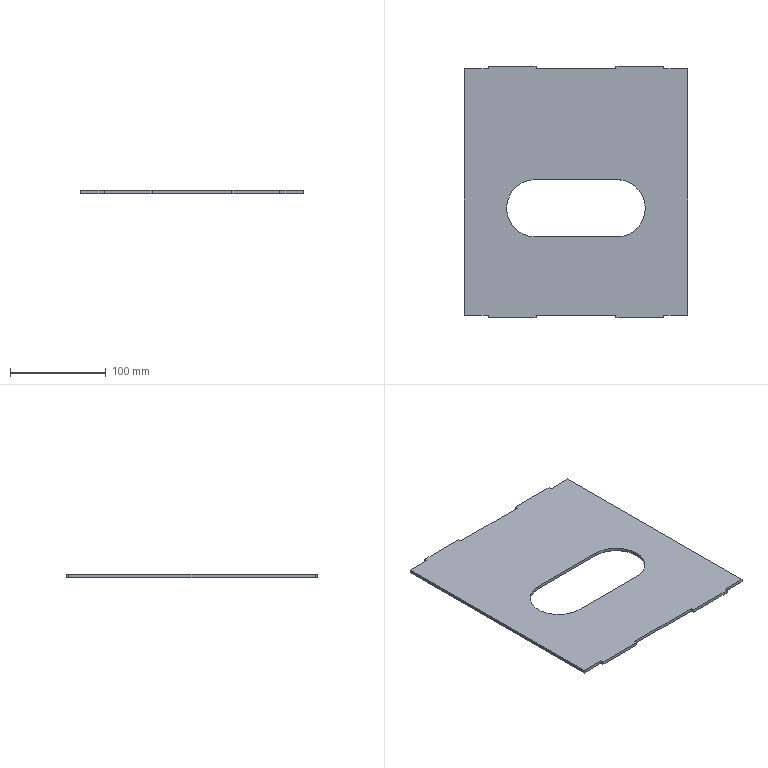Part | SolidWorks | features FlatPattern 1, SMBaseFlange 1, SheetMetal 1 | 1 solid | 27 faces | box 233.6 x 263.3 x 3.2 mm | volume 168889 mm3 | plane 24 | cylinder 3 | commonest cylinder face diameters 60 x3
STEP:
#1=CARTESIAN_POINT('',(-174.05,-276.65,-3.2));
#2=VERTEX_POINT('',#1);
#3=CARTESIAN_POINT('',(-204.05,-246.65,-3.2));
#4=VERTEX_POINT('',#3);
#5=CARTESIAN_POINT('',(-204.05,-276.65,-3.2));
#6=DIRECTION('',(0.,0.,1.));
#7=DIRECTION('',(1.,0.,0.));
#8=AXIS2_PLACEMENT_3D('',#5,#6,#7);
#9=CIRCLE('',#8,30.);
#10=EDGE_CURVE('',#2,#4,#9,.T.);
#11=ORIENTED_EDGE('',*,*,#10,.F.);
#12=CARTESIAN_POINT('',(-174.05,-276.65,0.));
#13=VERTEX_POINT('',#12);
#14=CARTESIAN_POINT('',(-174.05,-276.65,-3.2));
#15=DIRECTION('',(0.,0.,1.));
#16=VECTOR('',#15,1000.);
#17=LINE('',#14,#16);
#18=EDGE_CURVE('',#2,#13,#17,.T.);
#19=ORIENTED_EDGE('',*,*,#18,.T.);
#20=CARTESIAN_POINT('',(-204.05,-246.65,0.));
#21=VERTEX_POINT('',#20);
#22=CARTESIAN_POINT('',(-204.05,-276.65,0.));
#23=DIRECTION('',(0.,0.,1.));
#24=DIRECTION('',(1.,0.,0.));
#25=AXIS2_PLACEMENT_3D('',#22,#23,#24);
#26=CIRCLE('',#25,30.);
#27=EDGE_CURVE('',#13,#21,#26,.T.);
#28=ORIENTED_EDGE('',*,*,#27,.T.);
#29=CARTESIAN_POINT('',(-204.05,-246.65,-3.2));
#30=DIRECTION('',(0.,0.,1.));
#31=VECTOR('',#30,1000.);
#32=LINE('',#29,#31);
#33=EDGE_CURVE('',#4,#21,#32,.T.);
#34=ORIENTED_EDGE('',*,*,#33,.F.);
#35=EDGE_LOOP('',(#11,#19,#28,#34));
#36=FACE_OUTER_BOUND('',#35,.T.);
#37=CARTESIAN_POINT('',(-204.05,-276.65,-3.2));
#38=DIRECTION('',(0.,0.,1.));
#39=DIRECTION('',(1.,0.,0.));
#40=AXIS2_PLACEMENT_3D('',#37,#38,#39);
#41=CYLINDRICAL_SURFACE('',#40,30.);
#42=ADVANCED_FACE('',(#36),#41,.F.);
#43=CARTESIAN_POINT('',(-129.75,-388.35,0.));
#44=VERTEX_POINT('',#43);
#45=CARTESIAN_POINT('',(-129.75,-131.05,0.));
#46=VERTEX_POINT('',#45);
#47=CARTESIAN_POINT('',(-129.75,-388.35,0.));
#48=DIRECTION('',(0.,1.,0.));
#49=VECTOR('',#48,1000.);
#50=LINE('',#47,#49);
#51=EDGE_CURVE('',#44,#46,#50,.T.);
#52=ORIENTED_EDGE('',*,*,#51,.F.);
#53=CARTESIAN_POINT('',(-129.75,-388.35,-3.2));
#54=VERTEX_POINT('',#53);
#55=CARTESIAN_POINT('',(-129.75,-388.35,-3.2));
#56=DIRECTION('',(0.,0.,1.));
#57=VECTOR('',#56,1000.);
#58=LINE('',#55,#57);
#59=EDGE_CURVE('',#54,#44,#58,.T.);
#60=ORIENTED_EDGE('',*,*,#59,.F.);
#61=CARTESIAN_POINT('',(-129.75,-131.05,-3.2));
#62=VERTEX_POINT('',#61);
#63=CARTESIAN_POINT('',(-129.75,-388.35,-3.2));
#64=DIRECTION('',(0.,1.,0.));
#65=VECTOR('',#64,1000.);
#66=LINE('',#63,#65);
#67=EDGE_CURVE('',#54,#62,#66,.T.);
#68=ORIENTED_EDGE('',*,*,#67,.T.);
#69=CARTESIAN_POINT('',(-129.75,-131.05,-3.2));
#70=DIRECTION('',(0.,0.,1.));
#71=VECTOR('',#70,1000.);
#72=LINE('',#69,#71);
#73=EDGE_CURVE('',#62,#46,#72,.T.);
#74=ORIENTED_EDGE('',*,*,#73,.T.);
#75=EDGE_LOOP('',(#52,#60,#68,#74));
#76=FACE_OUTER_BOUND('',#75,.T.);
#77=CARTESIAN_POINT('',(-129.75,-388.35,-3.2));
#78=DIRECTION('',(1.,0.,0.));
#79=DIRECTION('',(0.,0.,-1.));
#80=AXIS2_PLACEMENT_3D('',#77,#78,#79);
#81=PLANE('',#80);
#82=ADVANCED_FACE('',(#76),#81,.T.);
#83=CARTESIAN_POINT('',(-154.75,-388.35,0.));
#84=VERTEX_POINT('',#83);
#85=CARTESIAN_POINT('',(-129.75,-388.35,0.));
#86=DIRECTION('',(1.,0.,0.));
#87=VECTOR('',#86,1000.);
#88=LINE('',#85,#87);
#89=EDGE_CURVE('',#84,#44,#88,.T.);
#90=ORIENTED_EDGE('',*,*,#89,.F.);
#91=CARTESIAN_POINT('',(-154.75,-388.35,-3.2));
#92=VERTEX_POINT('',#91);
#93=CARTESIAN_POINT('',(-154.75,-388.35,-3.2));
#94=DIRECTION('',(0.,0.,1.));
#95=VECTOR('',#94,1000.);
#96=LINE('',#93,#95);
#97=EDGE_CURVE('',#92,#84,#96,.T.);
#98=ORIENTED_EDGE('',*,*,#97,.F.);
#99=CARTESIAN_POINT('',(-129.75,-388.35,-3.2));
#100=DIRECTION('',(1.,0.,0.));
#101=VECTOR('',#100,1000.);
#102=LINE('',#99,#101);
#103=EDGE_CURVE('',#92,#54,#102,.T.);
#104=ORIENTED_EDGE('',*,*,#103,.T.);
#105=ORIENTED_EDGE('',*,*,#59,.T.);
#106=EDGE_LOOP('',(#90,#98,#104,#105));
#107=FACE_OUTER_BOUND('',#106,.T.);
#108=CARTESIAN_POINT('',(-129.75,-388.35,-3.2));
#109=DIRECTION('',(0.,-1.,0.));
#110=DIRECTION('',(0.,0.,-1.));
#111=AXIS2_PLACEMENT_3D('',#108,#109,#110);
#112=PLANE('',#111);
#113=ADVANCED_FACE('',(#107),#112,.T.);
#114=CARTESIAN_POINT('',(-154.75,-391.35,0.));
#115=VERTEX_POINT('',#114);
#116=CARTESIAN_POINT('',(-154.75,-388.35,0.));
#117=DIRECTION('',(0.,1.,0.));
#118=VECTOR('',#117,1000.);
#119=LINE('',#116,#118);
#120=EDGE_CURVE('',#115,#84,#119,.T.);
#121=ORIENTED_EDGE('',*,*,#120,.F.);
#122=CARTESIAN_POINT('',(-154.75,-391.35,-3.2));
#123=VERTEX_POINT('',#122);
#124=CARTESIAN_POINT('',(-154.75,-391.35,-3.2));
#125=DIRECTION('',(0.,0.,1.));
#126=VECTOR('',#125,1000.);
#127=LINE('',#124,#126);
#128=EDGE_CURVE('',#123,#115,#127,.T.);
#129=ORIENTED_EDGE('',*,*,#128,.F.);
#130=CARTESIAN_POINT('',(-154.75,-388.35,-3.2));
#131=DIRECTION('',(0.,1.,0.));
#132=VECTOR('',#131,1000.);
#133=LINE('',#130,#132);
#134=EDGE_CURVE('',#123,#92,#133,.T.);
#135=ORIENTED_EDGE('',*,*,#134,.T.);
#136=ORIENTED_EDGE('',*,*,#97,.T.);
#137=EDGE_LOOP('',(#121,#129,#135,#136));
#138=FACE_OUTER_BOUND('',#137,.T.);
#139=CARTESIAN_POINT('',(-154.75,-388.35,-3.2));
#140=DIRECTION('',(1.,0.,0.));
#141=DIRECTION('',(0.,0.,-1.));
#142=AXIS2_PLACEMENT_3D('',#139,#140,#141);
#143=PLANE('',#142);
#144=ADVANCED_FACE('',(#138),#143,.T.);
#145=CARTESIAN_POINT('',(-204.75,-391.35,0.));
#146=VERTEX_POINT('',#145);
#147=CARTESIAN_POINT('',(-154.75,-391.35,0.));
#148=DIRECTION('',(1.,0.,0.));
#149=VECTOR('',#148,1000.);
#150=LINE('',#147,#149);
#151=EDGE_CURVE('',#146,#115,#150,.T.);
#152=ORIENTED_EDGE('',*,*,#151,.F.);
#153=CARTESIAN_POINT('',(-204.75,-391.35,-3.2));
#154=VERTEX_POINT('',#153);
#155=CARTESIAN_POINT('',(-204.75,-391.35,-3.2));
#156=DIRECTION('',(0.,0.,1.));
#157=VECTOR('',#156,1000.);
#158=LINE('',#155,#157);
#159=EDGE_CURVE('',#154,#146,#158,.T.);
#160=ORIENTED_EDGE('',*,*,#159,.F.);
#161=CARTESIAN_POINT('',(-154.75,-391.35,-3.2));
#162=DIRECTION('',(1.,0.,0.));
#163=VECTOR('',#162,1000.);
#164=LINE('',#161,#163);
#165=EDGE_CURVE('',#154,#123,#164,.T.);
#166=ORIENTED_EDGE('',*,*,#165,.T.);
#167=ORIENTED_EDGE('',*,*,#128,.T.);
#168=EDGE_LOOP('',(#152,#160,#166,#167));
#169=FACE_OUTER_BOUND('',#168,.T.);
#170=CARTESIAN_POINT('',(-154.75,-391.35,-3.2));
#171=DIRECTION('',(0.,-1.,0.));
#172=DIRECTION('',(0.,0.,-1.));
#173=AXIS2_PLACEMENT_3D('',#170,#171,#172);
#174=PLANE('',#173);
#175=ADVANCED_FACE('',(#169),#174,.T.);
#176=CARTESIAN_POINT('',(-204.75,-388.35,0.));
#177=VERTEX_POINT('',#176);
#178=CARTESIAN_POINT('',(-204.75,-391.35,0.));
#179=DIRECTION('',(0.,-1.,0.));
#180=VECTOR('',#179,1000.);
#181=LINE('',#178,#180);
#182=EDGE_CURVE('',#177,#146,#181,.T.);
#183=ORIENTED_EDGE('',*,*,#182,.F.);
#184=CARTESIAN_POINT('',(-204.75,-388.35,-3.2));
#185=VERTEX_POINT('',#184);
#186=CARTESIAN_POINT('',(-204.75,-388.35,-3.2));
#187=DIRECTION('',(0.,0.,1.));
#188=VECTOR('',#187,1000.);
#189=LINE('',#186,#188);
#190=EDGE_CURVE('',#185,#177,#189,.T.);
#191=ORIENTED_EDGE('',*,*,#190,.F.);
#192=CARTESIAN_POINT('',(-204.75,-391.35,-3.2));
#193=DIRECTION('',(0.,-1.,0.));
#194=VECTOR('',#193,1000.);
#195=LINE('',#192,#194);
#196=EDGE_CURVE('',#185,#154,#195,.T.);
#197=ORIENTED_EDGE('',*,*,#196,.T.);
#198=ORIENTED_EDGE('',*,*,#159,.T.);
#199=EDGE_LOOP('',(#183,#191,#197,#198));
#200=FACE_OUTER_BOUND('',#199,.T.);
#201=CARTESIAN_POINT('',(-204.75,-391.35,-3.2));
#202=DIRECTION('',(-1.,0.,0.));
#203=DIRECTION('',(0.,0.,1.));
#204=AXIS2_PLACEMENT_3D('',#201,#202,#203);
#205=PLANE('',#204);
#206=ADVANCED_FACE('',(#200),#205,.T.);
#207=CARTESIAN_POINT('',(-288.35,-388.35,0.));
#208=VERTEX_POINT('',#207);
#209=CARTESIAN_POINT('',(-204.75,-388.35,0.));
#210=DIRECTION('',(1.,0.,0.));
#211=VECTOR('',#210,1000.);
#212=LINE('',#209,#211);
#213=EDGE_CURVE('',#208,#177,#212,.T.);
#214=ORIENTED_EDGE('',*,*,#213,.F.);
#215=CARTESIAN_POINT('',(-288.35,-388.35,-3.2));
#216=VERTEX_POINT('',#215);
#217=CARTESIAN_POINT('',(-288.35,-388.35,-3.2));
#218=DIRECTION('',(0.,0.,1.));
#219=VECTOR('',#218,1000.);
#220=LINE('',#217,#219);
#221=EDGE_CURVE('',#216,#208,#220,.T.);
#222=ORIENTED_EDGE('',*,*,#221,.F.);
#223=CARTESIAN_POINT('',(-204.75,-388.35,-3.2));
#224=DIRECTION('',(1.,0.,0.));
#225=VECTOR('',#224,1000.);
#226=LINE('',#223,#225);
#227=EDGE_CURVE('',#216,#185,#226,.T.);
#228=ORIENTED_EDGE('',*,*,#227,.T.);
#229=ORIENTED_EDGE('',*,*,#190,.T.);
#230=EDGE_LOOP('',(#214,#222,#228,#229));
#231=FACE_OUTER_BOUND('',#230,.T.);
#232=CARTESIAN_POINT('',(-204.75,-388.35,-3.2));
#233=DIRECTION('',(0.,-1.,0.));
#234=DIRECTION('',(0.,0.,-1.));
#235=AXIS2_PLACEMENT_3D('',#232,#233,#234);
#236=PLANE('',#235);
#237=ADVANCED_FACE('',(#231),#236,.T.);
#238=CARTESIAN_POINT('',(-288.35,-391.35,0.));
#239=VERTEX_POINT('',#238);
#240=CARTESIAN_POINT('',(-288.35,-391.35,0.));
#241=DIRECTION('',(0.,1.,0.));
#242=VECTOR('',#241,1000.);
#243=LINE('',#240,#242);
#244=EDGE_CURVE('',#239,#208,#243,.T.);
#245=ORIENTED_EDGE('',*,*,#244,.F.);
#246=CARTESIAN_POINT('',(-288.35,-391.35,-3.2));
#247=VERTEX_POINT('',#246);
#248=CARTESIAN_POINT('',(-288.35,-391.35,-3.2));
#249=DIRECTION('',(0.,0.,1.));
#250=VECTOR('',#249,1000.);
#251=LINE('',#248,#250);
#252=EDGE_CURVE('',#247,#239,#251,.T.);
#253=ORIENTED_EDGE('',*,*,#252,.F.);
#254=CARTESIAN_POINT('',(-288.35,-391.35,-3.2));
#255=DIRECTION('',(0.,1.,0.));
#256=VECTOR('',#255,1000.);
#257=LINE('',#254,#256);
#258=EDGE_CURVE('',#247,#216,#257,.T.);
#259=ORIENTED_EDGE('',*,*,#258,.T.);
#260=ORIENTED_EDGE('',*,*,#221,.T.);
#261=EDGE_LOOP('',(#245,#253,#259,#260));
#262=FACE_OUTER_BOUND('',#261,.T.);
#263=CARTESIAN_POINT('',(-288.35,-391.35,-3.2));
#264=DIRECTION('',(1.,0.,0.));
#265=DIRECTION('',(0.,0.,-1.));
#266=AXIS2_PLACEMENT_3D('',#263,#264,#265);
#267=PLANE('',#266);
#268=ADVANCED_FACE('',(#262),#267,.T.);
#269=CARTESIAN_POINT('',(-338.35,-391.35,0.));
#270=VERTEX_POINT('',#269);
#271=CARTESIAN_POINT('',(-338.35,-391.35,0.));
#272=DIRECTION('',(1.,0.,0.));
#273=VECTOR('',#272,1000.);
#274=LINE('',#271,#273);
#275=EDGE_CURVE('',#270,#239,#274,.T.);
#276=ORIENTED_EDGE('',*,*,#275,.F.);
#277=CARTESIAN_POINT('',(-338.35,-391.35,-3.2));
#278=VERTEX_POINT('',#277);
#279=CARTESIAN_POINT('',(-338.35,-391.35,-3.2));
#280=DIRECTION('',(0.,0.,1.));
#281=VECTOR('',#280,1000.);
#282=LINE('',#279,#281);
#283=EDGE_CURVE('',#278,#270,#282,.T.);
#284=ORIENTED_EDGE('',*,*,#283,.F.);
#285=CARTESIAN_POINT('',(-338.35,-391.35,-3.2));
#286=DIRECTION('',(1.,0.,0.));
#287=VECTOR('',#286,1000.);
#288=LINE('',#285,#287);
#289=EDGE_CURVE('',#278,#247,#288,.T.);
#290=ORIENTED_EDGE('',*,*,#289,.T.);
#291=ORIENTED_EDGE('',*,*,#252,.T.);
#292=EDGE_LOOP('',(#276,#284,#290,#291));
#293=FACE_OUTER_BOUND('',#292,.T.);
#294=CARTESIAN_POINT('',(-338.35,-391.35,-3.2));
#295=DIRECTION('',(0.,-1.,0.));
#296=DIRECTION('',(0.,0.,-1.));
#297=AXIS2_PLACEMENT_3D('',#294,#295,#296);
#298=PLANE('',#297);
#299=ADVANCED_FACE('',(#293),#298,.T.);
#300=CARTESIAN_POINT('',(-338.35,-388.35,0.));
#301=VERTEX_POINT('',#300);
#302=CARTESIAN_POINT('',(-338.35,-388.35,0.));
#303=DIRECTION('',(0.,-1.,0.));
#304=VECTOR('',#303,1000.);
#305=LINE('',#302,#304);
#306=EDGE_CURVE('',#301,#270,#305,.T.);
#307=ORIENTED_EDGE('',*,*,#306,.F.);
#308=CARTESIAN_POINT('',(-338.35,-388.35,-3.2));
#309=VERTEX_POINT('',#308);
#310=CARTESIAN_POINT('',(-338.35,-388.35,-3.2));
#311=DIRECTION('',(0.,0.,1.));
#312=VECTOR('',#311,1000.);
#313=LINE('',#310,#312);
#314=EDGE_CURVE('',#309,#301,#313,.T.);
#315=ORIENTED_EDGE('',*,*,#314,.F.);
#316=CARTESIAN_POINT('',(-338.35,-388.35,-3.2));
#317=DIRECTION('',(0.,-1.,0.));
#318=VECTOR('',#317,1000.);
#319=LINE('',#316,#318);
#320=EDGE_CURVE('',#309,#278,#319,.T.);
#321=ORIENTED_EDGE('',*,*,#320,.T.);
#322=ORIENTED_EDGE('',*,*,#283,.T.);
#323=EDGE_LOOP('',(#307,#315,#321,#322));
#324=FACE_OUTER_BOUND('',#323,.T.);
#325=CARTESIAN_POINT('',(-338.35,-388.35,-3.2));
#326=DIRECTION('',(-1.,0.,0.));
#327=DIRECTION('',(0.,0.,1.));
#328=AXIS2_PLACEMENT_3D('',#325,#326,#327);
#329=PLANE('',#328);
#330=ADVANCED_FACE('',(#324),#329,.T.);
#331=CARTESIAN_POINT('',(-363.35,-388.35,0.));
#332=VERTEX_POINT('',#331);
#333=CARTESIAN_POINT('',(-338.35,-388.35,0.));
#334=DIRECTION('',(1.,0.,0.));
#335=VECTOR('',#334,1000.);
#336=LINE('',#333,#335);
#337=EDGE_CURVE('',#332,#301,#336,.T.);
#338=ORIENTED_EDGE('',*,*,#337,.F.);
#339=CARTESIAN_POINT('',(-363.35,-388.35,-3.2));
#340=VERTEX_POINT('',#339);
#341=CARTESIAN_POINT('',(-363.35,-388.35,-3.2));
#342=DIRECTION('',(0.,0.,1.));
#343=VECTOR('',#342,1000.);
#344=LINE('',#341,#343);
#345=EDGE_CURVE('',#340,#332,#344,.T.);
#346=ORIENTED_EDGE('',*,*,#345,.F.);
#347=CARTESIAN_POINT('',(-338.35,-388.35,-3.2));
#348=DIRECTION('',(1.,0.,0.));
#349=VECTOR('',#348,1000.);
#350=LINE('',#347,#349);
#351=EDGE_CURVE('',#340,#309,#350,.T.);
#352=ORIENTED_EDGE('',*,*,#351,.T.);
#353=ORIENTED_EDGE('',*,*,#314,.T.);
#354=EDGE_LOOP('',(#338,#346,#352,#353));
#355=FACE_OUTER_BOUND('',#354,.T.);
#356=CARTESIAN_POINT('',(-338.35,-388.35,-3.2));
#357=DIRECTION('',(0.,-1.,0.));
#358=DIRECTION('',(0.,0.,-1.));
#359=AXIS2_PLACEMENT_3D('',#356,#357,#358);
#360=PLANE('',#359);
#361=ADVANCED_FACE('',(#355),#360,.T.);
#362=CARTESIAN_POINT('',(-363.35,-131.05,0.));
#363=VERTEX_POINT('',#362);
#364=CARTESIAN_POINT('',(-363.35,-388.35,0.));
#365=DIRECTION('',(0.,-1.,0.));
#366=VECTOR('',#365,1000.);
#367=LINE('',#364,#366);
#368=EDGE_CURVE('',#363,#332,#367,.T.);
#369=ORIENTED_EDGE('',*,*,#368,.F.);
#370=CARTESIAN_POINT('',(-363.35,-131.05,-3.2));
#371=VERTEX_POINT('',#370);
#372=CARTESIAN_POINT('',(-363.35,-131.05,-3.2));
#373=DIRECTION('',(0.,0.,1.));
#374=VECTOR('',#373,1000.);
#375=LINE('',#372,#374);
#376=EDGE_CURVE('',#371,#363,#375,.T.);
#377=ORIENTED_EDGE('',*,*,#376,.F.);
#378=CARTESIAN_POINT('',(-363.35,-388.35,-3.2));
#379=DIRECTION('',(0.,-1.,0.));
#380=VECTOR('',#379,1000.);
#381=LINE('',#378,#380);
#382=EDGE_CURVE('',#371,#340,#381,.T.);
#383=ORIENTED_EDGE('',*,*,#382,.T.);
#384=ORIENTED_EDGE('',*,*,#345,.T.);
#385=EDGE_LOOP('',(#369,#377,#383,#384));
#386=FACE_OUTER_BOUND('',#385,.T.);
#387=CARTESIAN_POINT('',(-363.35,-388.35,-3.2));
#388=DIRECTION('',(-1.,0.,0.));
#389=DIRECTION('',(0.,0.,1.));
#390=AXIS2_PLACEMENT_3D('',#387,#388,#389);
#391=PLANE('',#390);
#392=ADVANCED_FACE('',(#386),#391,.T.);
#393=CARTESIAN_POINT('',(-338.35,-131.05,0.));
#394=VERTEX_POINT('',#393);
#395=CARTESIAN_POINT('',(-338.35,-131.05,0.));
#396=DIRECTION('',(-1.,0.,0.));
#397=VECTOR('',#396,1000.);
#398=LINE('',#395,#397);
#399=EDGE_CURVE('',#394,#363,#398,.T.);
#400=ORIENTED_EDGE('',*,*,#399,.F.);
#401=CARTESIAN_POINT('',(-338.35,-131.05,-3.2));
#402=VERTEX_POINT('',#401);
#403=CARTESIAN_POINT('',(-338.35,-131.05,-3.2));
#404=DIRECTION('',(0.,0.,1.));
#405=VECTOR('',#404,1000.);
#406=LINE('',#403,#405);
#407=EDGE_CURVE('',#402,#394,#406,.T.);
#408=ORIENTED_EDGE('',*,*,#407,.F.);
#409=CARTESIAN_POINT('',(-338.35,-131.05,-3.2));
#410=DIRECTION('',(-1.,0.,0.));
#411=VECTOR('',#410,1000.);
#412=LINE('',#409,#411);
#413=EDGE_CURVE('',#402,#371,#412,.T.);
#414=ORIENTED_EDGE('',*,*,#413,.T.);
#415=ORIENTED_EDGE('',*,*,#376,.T.);
#416=EDGE_LOOP('',(#400,#408,#414,#415));
#417=FACE_OUTER_BOUND('',#416,.T.);
#418=CARTESIAN_POINT('',(-338.35,-131.05,-3.2));
#419=DIRECTION('',(0.,1.,0.));
#420=DIRECTION('',(0.,0.,1.));
#421=AXIS2_PLACEMENT_3D('',#418,#419,#420);
#422=PLANE('',#421);
#423=ADVANCED_FACE('',(#417),#422,.T.);
#424=CARTESIAN_POINT('',(-338.35,-128.05,0.));
#425=VERTEX_POINT('',#424);
#426=CARTESIAN_POINT('',(-338.35,-131.05,0.));
#427=DIRECTION('',(0.,-1.,0.));
#428=VECTOR('',#427,1000.);
#429=LINE('',#426,#428);
#430=EDGE_CURVE('',#425,#394,#429,.T.);
#431=ORIENTED_EDGE('',*,*,#430,.F.);
#432=CARTESIAN_POINT('',(-338.35,-128.05,-3.2));
#433=VERTEX_POINT('',#432);
#434=CARTESIAN_POINT('',(-338.35,-128.05,-3.2));
#435=DIRECTION('',(0.,0.,1.));
#436=VECTOR('',#435,1000.);
#437=LINE('',#434,#436);
#438=EDGE_CURVE('',#433,#425,#437,.T.);
#439=ORIENTED_EDGE('',*,*,#438,.F.);
#440=CARTESIAN_POINT('',(-338.35,-131.05,-3.2));
#441=DIRECTION('',(0.,-1.,0.));
#442=VECTOR('',#441,1000.);
#443=LINE('',#440,#442);
#444=EDGE_CURVE('',#433,#402,#443,.T.);
#445=ORIENTED_EDGE('',*,*,#444,.T.);
#446=ORIENTED_EDGE('',*,*,#407,.T.);
#447=EDGE_LOOP('',(#431,#439,#445,#446));
#448=FACE_OUTER_BOUND('',#447,.T.);
#449=CARTESIAN_POINT('',(-338.35,-131.05,-3.2));
#450=DIRECTION('',(-1.,0.,0.));
#451=DIRECTION('',(0.,0.,1.));
#452=AXIS2_PLACEMENT_3D('',#449,#450,#451);
#453=PLANE('',#452);
#454=ADVANCED_FACE('',(#448),#453,.T.);
#455=CARTESIAN_POINT('',(-288.35,-128.05,0.));
#456=VERTEX_POINT('',#455);
#457=CARTESIAN_POINT('',(-338.35,-128.05,0.));
#458=DIRECTION('',(-1.,0.,0.));
#459=VECTOR('',#458,1000.);
#460=LINE('',#457,#459);
#461=EDGE_CURVE('',#456,#425,#460,.T.);
#462=ORIENTED_EDGE('',*,*,#461,.F.);
#463=CARTESIAN_POINT('',(-288.35,-128.05,-3.2));
#464=VERTEX_POINT('',#463);
#465=CARTESIAN_POINT('',(-288.35,-128.05,-3.2));
#466=DIRECTION('',(0.,0.,1.));
#467=VECTOR('',#466,1000.);
#468=LINE('',#465,#467);
#469=EDGE_CURVE('',#464,#456,#468,.T.);
#470=ORIENTED_EDGE('',*,*,#469,.F.);
#471=CARTESIAN_POINT('',(-338.35,-128.05,-3.2));
#472=DIRECTION('',(-1.,0.,0.));
#473=VECTOR('',#472,1000.);
#474=LINE('',#471,#473);
#475=EDGE_CURVE('',#464,#433,#474,.T.);
#476=ORIENTED_EDGE('',*,*,#475,.T.);
#477=ORIENTED_EDGE('',*,*,#438,.T.);
#478=EDGE_LOOP('',(#462,#470,#476,#477));
#479=FACE_OUTER_BOUND('',#478,.T.);
#480=CARTESIAN_POINT('',(-338.35,-128.05,-3.2));
#481=DIRECTION('',(0.,1.,0.));
#482=DIRECTION('',(0.,0.,1.));
#483=AXIS2_PLACEMENT_3D('',#480,#481,#482);
#484=PLANE('',#483);
#485=ADVANCED_FACE('',(#479),#484,.T.);
#486=CARTESIAN_POINT('',(-288.35,-131.05,0.));
#487=VERTEX_POINT('',#486);
#488=CARTESIAN_POINT('',(-288.35,-128.05,0.));
#489=DIRECTION('',(0.,1.,0.));
#490=VECTOR('',#489,1000.);
#491=LINE('',#488,#490);
#492=EDGE_CURVE('',#487,#456,#491,.T.);
#493=ORIENTED_EDGE('',*,*,#492,.F.);
#494=CARTESIAN_POINT('',(-288.35,-131.05,-3.2));
#495=VERTEX_POINT('',#494);
#496=CARTESIAN_POINT('',(-288.35,-131.05,-3.2));
#497=DIRECTION('',(0.,0.,1.));
#498=VECTOR('',#497,1000.);
#499=LINE('',#496,#498);
#500=EDGE_CURVE('',#495,#487,#499,.T.);
#501=ORIENTED_EDGE('',*,*,#500,.F.);
#502=CARTESIAN_POINT('',(-288.35,-128.05,-3.2));
#503=DIRECTION('',(0.,1.,0.));
#504=VECTOR('',#503,1000.);
#505=LINE('',#502,#504);
#506=EDGE_CURVE('',#495,#464,#505,.T.);
#507=ORIENTED_EDGE('',*,*,#506,.T.);
#508=ORIENTED_EDGE('',*,*,#469,.T.);
#509=EDGE_LOOP('',(#493,#501,#507,#508));
#510=FACE_OUTER_BOUND('',#509,.T.);
#511=CARTESIAN_POINT('',(-288.35,-128.05,-3.2));
#512=DIRECTION('',(1.,0.,0.));
#513=DIRECTION('',(0.,0.,-1.));
#514=AXIS2_PLACEMENT_3D('',#511,#512,#513);
#515=PLANE('',#514);
#516=ADVANCED_FACE('',(#510),#515,.T.);
#517=CARTESIAN_POINT('',(-204.75,-131.05,0.));
#518=VERTEX_POINT('',#517);
#519=CARTESIAN_POINT('',(-204.75,-131.05,0.));
#520=DIRECTION('',(-1.,0.,0.));
#521=VECTOR('',#520,1000.);
#522=LINE('',#519,#521);
#523=EDGE_CURVE('',#518,#487,#522,.T.);
#524=ORIENTED_EDGE('',*,*,#523,.F.);
#525=CARTESIAN_POINT('',(-204.75,-131.05,-3.2));
#526=VERTEX_POINT('',#525);
#527=CARTESIAN_POINT('',(-204.75,-131.05,-3.2));
#528=DIRECTION('',(0.,0.,1.));
#529=VECTOR('',#528,1000.);
#530=LINE('',#527,#529);
#531=EDGE_CURVE('',#526,#518,#530,.T.);
#532=ORIENTED_EDGE('',*,*,#531,.F.);
#533=CARTESIAN_POINT('',(-204.75,-131.05,-3.2));
#534=DIRECTION('',(-1.,0.,0.));
#535=VECTOR('',#534,1000.);
#536=LINE('',#533,#535);
#537=EDGE_CURVE('',#526,#495,#536,.T.);
#538=ORIENTED_EDGE('',*,*,#537,.T.);
#539=ORIENTED_EDGE('',*,*,#500,.T.);
#540=EDGE_LOOP('',(#524,#532,#538,#539));
#541=FACE_OUTER_BOUND('',#540,.T.);
#542=CARTESIAN_POINT('',(-204.75,-131.05,-3.2));
#543=DIRECTION('',(0.,1.,0.));
#544=DIRECTION('',(-1.,0.,0.));
#545=AXIS2_PLACEMENT_3D('',#542,#543,#544);
#546=PLANE('',#545);
#547=ADVANCED_FACE('',(#541),#546,.T.);
#548=CARTESIAN_POINT('',(-204.75,-128.05,0.));
#549=VERTEX_POINT('',#548);
#550=CARTESIAN_POINT('',(-204.75,-128.05,0.));
#551=DIRECTION('',(0.,-1.,0.));
#552=VECTOR('',#551,1000.);
#553=LINE('',#550,#552);
#554=EDGE_CURVE('',#549,#518,#553,.T.);
#555=ORIENTED_EDGE('',*,*,#554,.F.);
#556=CARTESIAN_POINT('',(-204.75,-128.05,-3.2));
#557=VERTEX_POINT('',#556);
#558=CARTESIAN_POINT('',(-204.75,-128.05,-3.2));
#559=DIRECTION('',(0.,0.,1.));
#560=VECTOR('',#559,1000.);
#561=LINE('',#558,#560);
#562=EDGE_CURVE('',#557,#549,#561,.T.);
#563=ORIENTED_EDGE('',*,*,#562,.F.);
#564=CARTESIAN_POINT('',(-204.75,-128.05,-3.2));
#565=DIRECTION('',(0.,-1.,0.));
#566=VECTOR('',#565,1000.);
#567=LINE('',#564,#566);
#568=EDGE_CURVE('',#557,#526,#567,.T.);
#569=ORIENTED_EDGE('',*,*,#568,.T.);
#570=ORIENTED_EDGE('',*,*,#531,.T.);
#571=EDGE_LOOP('',(#555,#563,#569,#570));
#572=FACE_OUTER_BOUND('',#571,.T.);
#573=CARTESIAN_POINT('',(-204.75,-128.05,-3.2));
#574=DIRECTION('',(-1.,0.,0.));
#575=DIRECTION('',(0.,0.,1.));
#576=AXIS2_PLACEMENT_3D('',#573,#574,#575);
#577=PLANE('',#576);
#578=ADVANCED_FACE('',(#572),#577,.T.);
#579=CARTESIAN_POINT('',(-154.75,-128.05,0.));
#580=VERTEX_POINT('',#579);
#581=CARTESIAN_POINT('',(-154.75,-128.05,0.));
#582=DIRECTION('',(-1.,0.,0.));
#583=VECTOR('',#582,1000.);
#584=LINE('',#581,#583);
#585=EDGE_CURVE('',#580,#549,#584,.T.);
#586=ORIENTED_EDGE('',*,*,#585,.F.);
#587=CARTESIAN_POINT('',(-154.75,-128.05,-3.2));
#588=VERTEX_POINT('',#587);
#589=CARTESIAN_POINT('',(-154.75,-128.05,-3.2));
#590=DIRECTION('',(0.,0.,1.));
#591=VECTOR('',#590,1000.);
#592=LINE('',#589,#591);
#593=EDGE_CURVE('',#588,#580,#592,.T.);
#594=ORIENTED_EDGE('',*,*,#593,.F.);
#595=CARTESIAN_POINT('',(-154.75,-128.05,-3.2));
#596=DIRECTION('',(-1.,0.,0.));
#597=VECTOR('',#596,1000.);
#598=LINE('',#595,#597);
#599=EDGE_CURVE('',#588,#557,#598,.T.);
#600=ORIENTED_EDGE('',*,*,#599,.T.);
#601=ORIENTED_EDGE('',*,*,#562,.T.);
#602=EDGE_LOOP('',(#586,#594,#600,#601));
#603=FACE_OUTER_BOUND('',#602,.T.);
#604=CARTESIAN_POINT('',(-154.75,-128.05,-3.2));
#605=DIRECTION('',(0.,1.,0.));
#606=DIRECTION('',(-1.,0.,0.));
#607=AXIS2_PLACEMENT_3D('',#604,#605,#606);
#608=PLANE('',#607);
#609=ADVANCED_FACE('',(#603),#608,.T.);
#610=CARTESIAN_POINT('',(-154.75,-131.05,0.));
#611=VERTEX_POINT('',#610);
#612=CARTESIAN_POINT('',(-154.75,-131.05,0.));
#613=DIRECTION('',(0.,1.,0.));
#614=VECTOR('',#613,1000.);
#615=LINE('',#612,#614);
#616=EDGE_CURVE('',#611,#580,#615,.T.);
#617=ORIENTED_EDGE('',*,*,#616,.F.);
#618=CARTESIAN_POINT('',(-154.75,-131.05,-3.2));
#619=VERTEX_POINT('',#618);
#620=CARTESIAN_POINT('',(-154.75,-131.05,-3.2));
#621=DIRECTION('',(0.,0.,1.));
#622=VECTOR('',#621,1000.);
#623=LINE('',#620,#622);
#624=EDGE_CURVE('',#619,#611,#623,.T.);
#625=ORIENTED_EDGE('',*,*,#624,.F.);
#626=CARTESIAN_POINT('',(-154.75,-131.05,-3.2));
#627=DIRECTION('',(0.,1.,0.));
#628=VECTOR('',#627,1000.);
#629=LINE('',#626,#628);
#630=EDGE_CURVE('',#619,#588,#629,.T.);
#631=ORIENTED_EDGE('',*,*,#630,.T.);
#632=ORIENTED_EDGE('',*,*,#593,.T.);
#633=EDGE_LOOP('',(#617,#625,#631,#632));
#634=FACE_OUTER_BOUND('',#633,.T.);
#635=CARTESIAN_POINT('',(-154.75,-131.05,-3.2));
#636=DIRECTION('',(1.,0.,0.));
#637=DIRECTION('',(0.,0.,-1.));
#638=AXIS2_PLACEMENT_3D('',#635,#636,#637);
#639=PLANE('',#638);
#640=ADVANCED_FACE('',(#634),#639,.T.);
#641=CARTESIAN_POINT('',(-129.75,-131.05,0.));
#642=DIRECTION('',(-1.,0.,0.));
#643=VECTOR('',#642,1000.);
#644=LINE('',#641,#643);
#645=EDGE_CURVE('',#46,#611,#644,.T.);
#646=ORIENTED_EDGE('',*,*,#645,.F.);
#647=ORIENTED_EDGE('',*,*,#73,.F.);
#648=CARTESIAN_POINT('',(-129.75,-131.05,-3.2));
#649=DIRECTION('',(-1.,0.,0.));
#650=VECTOR('',#649,1000.);
#651=LINE('',#648,#650);
#652=EDGE_CURVE('',#62,#619,#651,.T.);
#653=ORIENTED_EDGE('',*,*,#652,.T.);
#654=ORIENTED_EDGE('',*,*,#624,.T.);
#655=EDGE_LOOP('',(#646,#647,#653,#654));
#656=FACE_OUTER_BOUND('',#655,.T.);
#657=CARTESIAN_POINT('',(-129.75,-131.05,-3.2));
#658=DIRECTION('',(0.,1.,0.));
#659=DIRECTION('',(-1.,0.,0.));
#660=AXIS2_PLACEMENT_3D('',#657,#658,#659);
#661=PLANE('',#660);
#662=ADVANCED_FACE('',(#656),#661,.T.);
#663=CARTESIAN_POINT('',(-289.05,-306.65,-3.2));
#664=VERTEX_POINT('',#663);
#665=CARTESIAN_POINT('',(-204.05,-306.65,-3.2));
#666=VERTEX_POINT('',#665);
#667=CARTESIAN_POINT('',(-204.05,-306.65,-3.2));
#668=DIRECTION('',(1.,0.,0.));
#669=VECTOR('',#668,1000.);
#670=LINE('',#667,#669);
#671=EDGE_CURVE('',#664,#666,#670,.T.);
#672=ORIENTED_EDGE('',*,*,#671,.T.);
#673=CARTESIAN_POINT('',(-204.05,-276.65,-3.2));
#674=DIRECTION('',(0.,0.,1.));
#675=DIRECTION('',(1.,0.,0.));
#676=AXIS2_PLACEMENT_3D('',#673,#674,#675);
#677=CIRCLE('',#676,30.);
#678=EDGE_CURVE('',#666,#2,#677,.T.);
#679=ORIENTED_EDGE('',*,*,#678,.T.);
#680=ORIENTED_EDGE('',*,*,#10,.T.);
#681=CARTESIAN_POINT('',(-289.05,-246.65,-3.2));
#682=VERTEX_POINT('',#681);
#683=CARTESIAN_POINT('',(-204.05,-246.65,-3.2));
#684=DIRECTION('',(-1.,0.,0.));
#685=VECTOR('',#684,1000.);
#686=LINE('',#683,#685);
#687=EDGE_CURVE('',#4,#682,#686,.T.);
#688=ORIENTED_EDGE('',*,*,#687,.T.);
#689=CARTESIAN_POINT('',(-289.05,-276.65,-3.2));
#690=DIRECTION('',(0.,0.,1.));
#691=DIRECTION('',(1.,0.,0.));
#692=AXIS2_PLACEMENT_3D('',#689,#690,#691);
#693=CIRCLE('',#692,30.);
#694=EDGE_CURVE('',#682,#664,#693,.T.);
#695=ORIENTED_EDGE('',*,*,#694,.T.);
#696=EDGE_LOOP('',(#672,#679,#680,#688,#695));
#697=FACE_BOUND('',#696,.T.);
#698=ORIENTED_EDGE('',*,*,#67,.F.);
#699=ORIENTED_EDGE('',*,*,#103,.F.);
#700=ORIENTED_EDGE('',*,*,#134,.F.);
#701=ORIENTED_EDGE('',*,*,#165,.F.);
#702=ORIENTED_EDGE('',*,*,#196,.F.);
#703=ORIENTED_EDGE('',*,*,#227,.F.);
#704=ORIENTED_EDGE('',*,*,#258,.F.);
#705=ORIENTED_EDGE('',*,*,#289,.F.);
#706=ORIENTED_EDGE('',*,*,#320,.F.);
#707=ORIENTED_EDGE('',*,*,#351,.F.);
#708=ORIENTED_EDGE('',*,*,#382,.F.);
#709=ORIENTED_EDGE('',*,*,#413,.F.);
#710=ORIENTED_EDGE('',*,*,#444,.F.);
#711=ORIENTED_EDGE('',*,*,#475,.F.);
#712=ORIENTED_EDGE('',*,*,#506,.F.);
#713=ORIENTED_EDGE('',*,*,#537,.F.);
#714=ORIENTED_EDGE('',*,*,#568,.F.);
#715=ORIENTED_EDGE('',*,*,#599,.F.);
#716=ORIENTED_EDGE('',*,*,#630,.F.);
#717=ORIENTED_EDGE('',*,*,#652,.F.);
#718=EDGE_LOOP('',(#698,#699,#700,#701,#702,#703,#704,#705,#706,#707,#708,#709,#710,#711,#712,#713,#714,#715,#716,#717));
#719=FACE_OUTER_BOUND('',#718,.T.);
#720=CARTESIAN_POINT('',(0.,0.,-3.2));
#721=DIRECTION('',(0.,0.,1.));
#722=DIRECTION('',(1.,0.,0.));
#723=AXIS2_PLACEMENT_3D('',#720,#721,#722);
#724=PLANE('',#723);
#725=ADVANCED_FACE('',(#697,#719),#724,.F.);
#726=CARTESIAN_POINT('',(-204.05,-306.65,0.));
#727=VERTEX_POINT('',#726);
#728=CARTESIAN_POINT('',(-204.05,-276.65,0.));
#729=DIRECTION('',(0.,0.,1.));
#730=DIRECTION('',(1.,0.,0.));
#731=AXIS2_PLACEMENT_3D('',#728,#729,#730);
#732=CIRCLE('',#731,30.);
#733=EDGE_CURVE('',#727,#13,#732,.T.);
#734=ORIENTED_EDGE('',*,*,#733,.F.);
#735=CARTESIAN_POINT('',(-289.05,-306.65,0.));
#736=VERTEX_POINT('',#735);
#737=CARTESIAN_POINT('',(-204.05,-306.65,0.));
#738=DIRECTION('',(1.,0.,0.));
#739=VECTOR('',#738,1000.);
#740=LINE('',#737,#739);
#741=EDGE_CURVE('',#736,#727,#740,.T.);
#742=ORIENTED_EDGE('',*,*,#741,.F.);
#743=CARTESIAN_POINT('',(-289.05,-246.65,0.));
#744=VERTEX_POINT('',#743);
#745=CARTESIAN_POINT('',(-289.05,-276.65,0.));
#746=DIRECTION('',(0.,0.,1.));
#747=DIRECTION('',(1.,0.,0.));
#748=AXIS2_PLACEMENT_3D('',#745,#746,#747);
#749=CIRCLE('',#748,30.);
#750=EDGE_CURVE('',#744,#736,#749,.T.);
#751=ORIENTED_EDGE('',*,*,#750,.F.);
#752=CARTESIAN_POINT('',(-204.05,-246.65,0.));
#753=DIRECTION('',(-1.,0.,0.));
#754=VECTOR('',#753,1000.);
#755=LINE('',#752,#754);
#756=EDGE_CURVE('',#21,#744,#755,.T.);
#757=ORIENTED_EDGE('',*,*,#756,.F.);
#758=ORIENTED_EDGE('',*,*,#27,.F.);
#759=EDGE_LOOP('',(#734,#742,#751,#757,#758));
#760=FACE_BOUND('',#759,.T.);
#761=ORIENTED_EDGE('',*,*,#51,.T.);
#762=ORIENTED_EDGE('',*,*,#645,.T.);
#763=ORIENTED_EDGE('',*,*,#616,.T.);
#764=ORIENTED_EDGE('',*,*,#585,.T.);
#765=ORIENTED_EDGE('',*,*,#554,.T.);
#766=ORIENTED_EDGE('',*,*,#523,.T.);
#767=ORIENTED_EDGE('',*,*,#492,.T.);
#768=ORIENTED_EDGE('',*,*,#461,.T.);
#769=ORIENTED_EDGE('',*,*,#430,.T.);
#770=ORIENTED_EDGE('',*,*,#399,.T.);
#771=ORIENTED_EDGE('',*,*,#368,.T.);
#772=ORIENTED_EDGE('',*,*,#337,.T.);
#773=ORIENTED_EDGE('',*,*,#306,.T.);
#774=ORIENTED_EDGE('',*,*,#275,.T.);
#775=ORIENTED_EDGE('',*,*,#244,.T.);
#776=ORIENTED_EDGE('',*,*,#213,.T.);
#777=ORIENTED_EDGE('',*,*,#182,.T.);
#778=ORIENTED_EDGE('',*,*,#151,.T.);
#779=ORIENTED_EDGE('',*,*,#120,.T.);
#780=ORIENTED_EDGE('',*,*,#89,.T.);
#781=EDGE_LOOP('',(#761,#762,#763,#764,#765,#766,#767,#768,#769,#770,#771,#772,#773,#774,#775,#776,#777,#778,#779,#780));
#782=FACE_OUTER_BOUND('',#781,.T.);
#783=CARTESIAN_POINT('',(0.,0.,0.));
#784=DIRECTION('',(0.,0.,1.));
#785=DIRECTION('',(1.,0.,0.));
#786=AXIS2_PLACEMENT_3D('',#783,#784,#785);
#787=PLANE('',#786);
#788=ADVANCED_FACE('',(#760,#782),#787,.T.);
#789=ORIENTED_EDGE('',*,*,#18,.F.);
#790=ORIENTED_EDGE('',*,*,#678,.F.);
#791=CARTESIAN_POINT('',(-204.05,-306.65,-3.2));
#792=DIRECTION('',(0.,0.,1.));
#793=VECTOR('',#792,1000.);
#794=LINE('',#791,#793);
#795=EDGE_CURVE('',#666,#727,#794,.T.);
#796=ORIENTED_EDGE('',*,*,#795,.T.);
#797=ORIENTED_EDGE('',*,*,#733,.T.);
#798=EDGE_LOOP('',(#789,#790,#796,#797));
#799=FACE_OUTER_BOUND('',#798,.T.);
#800=CARTESIAN_POINT('',(-204.05,-276.65,-3.2));
#801=DIRECTION('',(0.,0.,1.));
#802=DIRECTION('',(1.,0.,0.));
#803=AXIS2_PLACEMENT_3D('',#800,#801,#802);
#804=CYLINDRICAL_SURFACE('',#803,30.);
#805=ADVANCED_FACE('',(#799),#804,.F.);
#806=ORIENTED_EDGE('',*,*,#741,.T.);
#807=ORIENTED_EDGE('',*,*,#795,.F.);
#808=ORIENTED_EDGE('',*,*,#671,.F.);
#809=CARTESIAN_POINT('',(-289.05,-306.65,-3.2));
#810=DIRECTION('',(0.,0.,1.));
#811=VECTOR('',#810,1000.);
#812=LINE('',#809,#811);
#813=EDGE_CURVE('',#664,#736,#812,.T.);
#814=ORIENTED_EDGE('',*,*,#813,.T.);
#815=EDGE_LOOP('',(#806,#807,#808,#814));
#816=FACE_OUTER_BOUND('',#815,.T.);
#817=CARTESIAN_POINT('',(-204.05,-306.65,-3.2));
#818=DIRECTION('',(0.,-1.,0.));
#819=DIRECTION('',(0.,0.,-1.));
#820=AXIS2_PLACEMENT_3D('',#817,#818,#819);
#821=PLANE('',#820);
#822=ADVANCED_FACE('',(#816),#821,.F.);
#823=ORIENTED_EDGE('',*,*,#750,.T.);
#824=ORIENTED_EDGE('',*,*,#813,.F.);
#825=ORIENTED_EDGE('',*,*,#694,.F.);
#826=CARTESIAN_POINT('',(-289.05,-246.65,-3.2));
#827=DIRECTION('',(0.,0.,1.));
#828=VECTOR('',#827,1000.);
#829=LINE('',#826,#828);
#830=EDGE_CURVE('',#682,#744,#829,.T.);
#831=ORIENTED_EDGE('',*,*,#830,.T.);
#832=EDGE_LOOP('',(#823,#824,#825,#831));
#833=FACE_OUTER_BOUND('',#832,.T.);
#834=CARTESIAN_POINT('',(-289.05,-276.65,-3.2));
#835=DIRECTION('',(0.,0.,1.));
#836=DIRECTION('',(1.,0.,0.));
#837=AXIS2_PLACEMENT_3D('',#834,#835,#836);
#838=CYLINDRICAL_SURFACE('',#837,30.);
#839=ADVANCED_FACE('',(#833),#838,.F.);
#840=ORIENTED_EDGE('',*,*,#756,.T.);
#841=ORIENTED_EDGE('',*,*,#830,.F.);
#842=ORIENTED_EDGE('',*,*,#687,.F.);
#843=ORIENTED_EDGE('',*,*,#33,.T.);
#844=EDGE_LOOP('',(#840,#841,#842,#843));
#845=FACE_OUTER_BOUND('',#844,.T.);
#846=CARTESIAN_POINT('',(-204.05,-246.65,-3.2));
#847=DIRECTION('',(0.,1.,0.));
#848=DIRECTION('',(0.,0.,1.));
#849=AXIS2_PLACEMENT_3D('',#846,#847,#848);
#850=PLANE('',#849);
#851=ADVANCED_FACE('',(#845),#850,.F.);
#852=CLOSED_SHELL('',(#42,#82,#113,#144,#175,#206,#237,#268,#299,#330,#361,#392,#423,#454,#485,#516,#547,#578,#609,#640,#662,#725,#788,#805,#822,#839,#851));
#853=MANIFOLD_SOLID_BREP('',#852);
#854=CARTESIAN_POINT('',(0.,0.,0.));
#855=DIRECTION('',(0.,0.,1.));
#856=DIRECTION('',(1.,0.,0.));
#857=AXIS2_PLACEMENT_3D('',#854,#855,#856);
#858=(LENGTH_UNIT()NAMED_UNIT(*)SI_UNIT(.MILLI.,.METRE.));
#859=UNCERTAINTY_MEASURE_WITH_UNIT(LENGTH_MEASURE(0.00001),#858,'','');
#860=(NAMED_UNIT(*)PLANE_ANGLE_UNIT()SI_UNIT($,.RADIAN.));
#861=(NAMED_UNIT(*)SI_UNIT($,.STERADIAN.)SOLID_ANGLE_UNIT());
#862=(GEOMETRIC_REPRESENTATION_CONTEXT(3)GLOBAL_UNCERTAINTY_ASSIGNED_CONTEXT((#859))GLOBAL_UNIT_ASSIGNED_CONTEXT((#858,#860,#861))REPRESENTATION_CONTEXT('',''));
#863=ADVANCED_BREP_SHAPE_REPRESENTATION('',(#853,#857),#862);